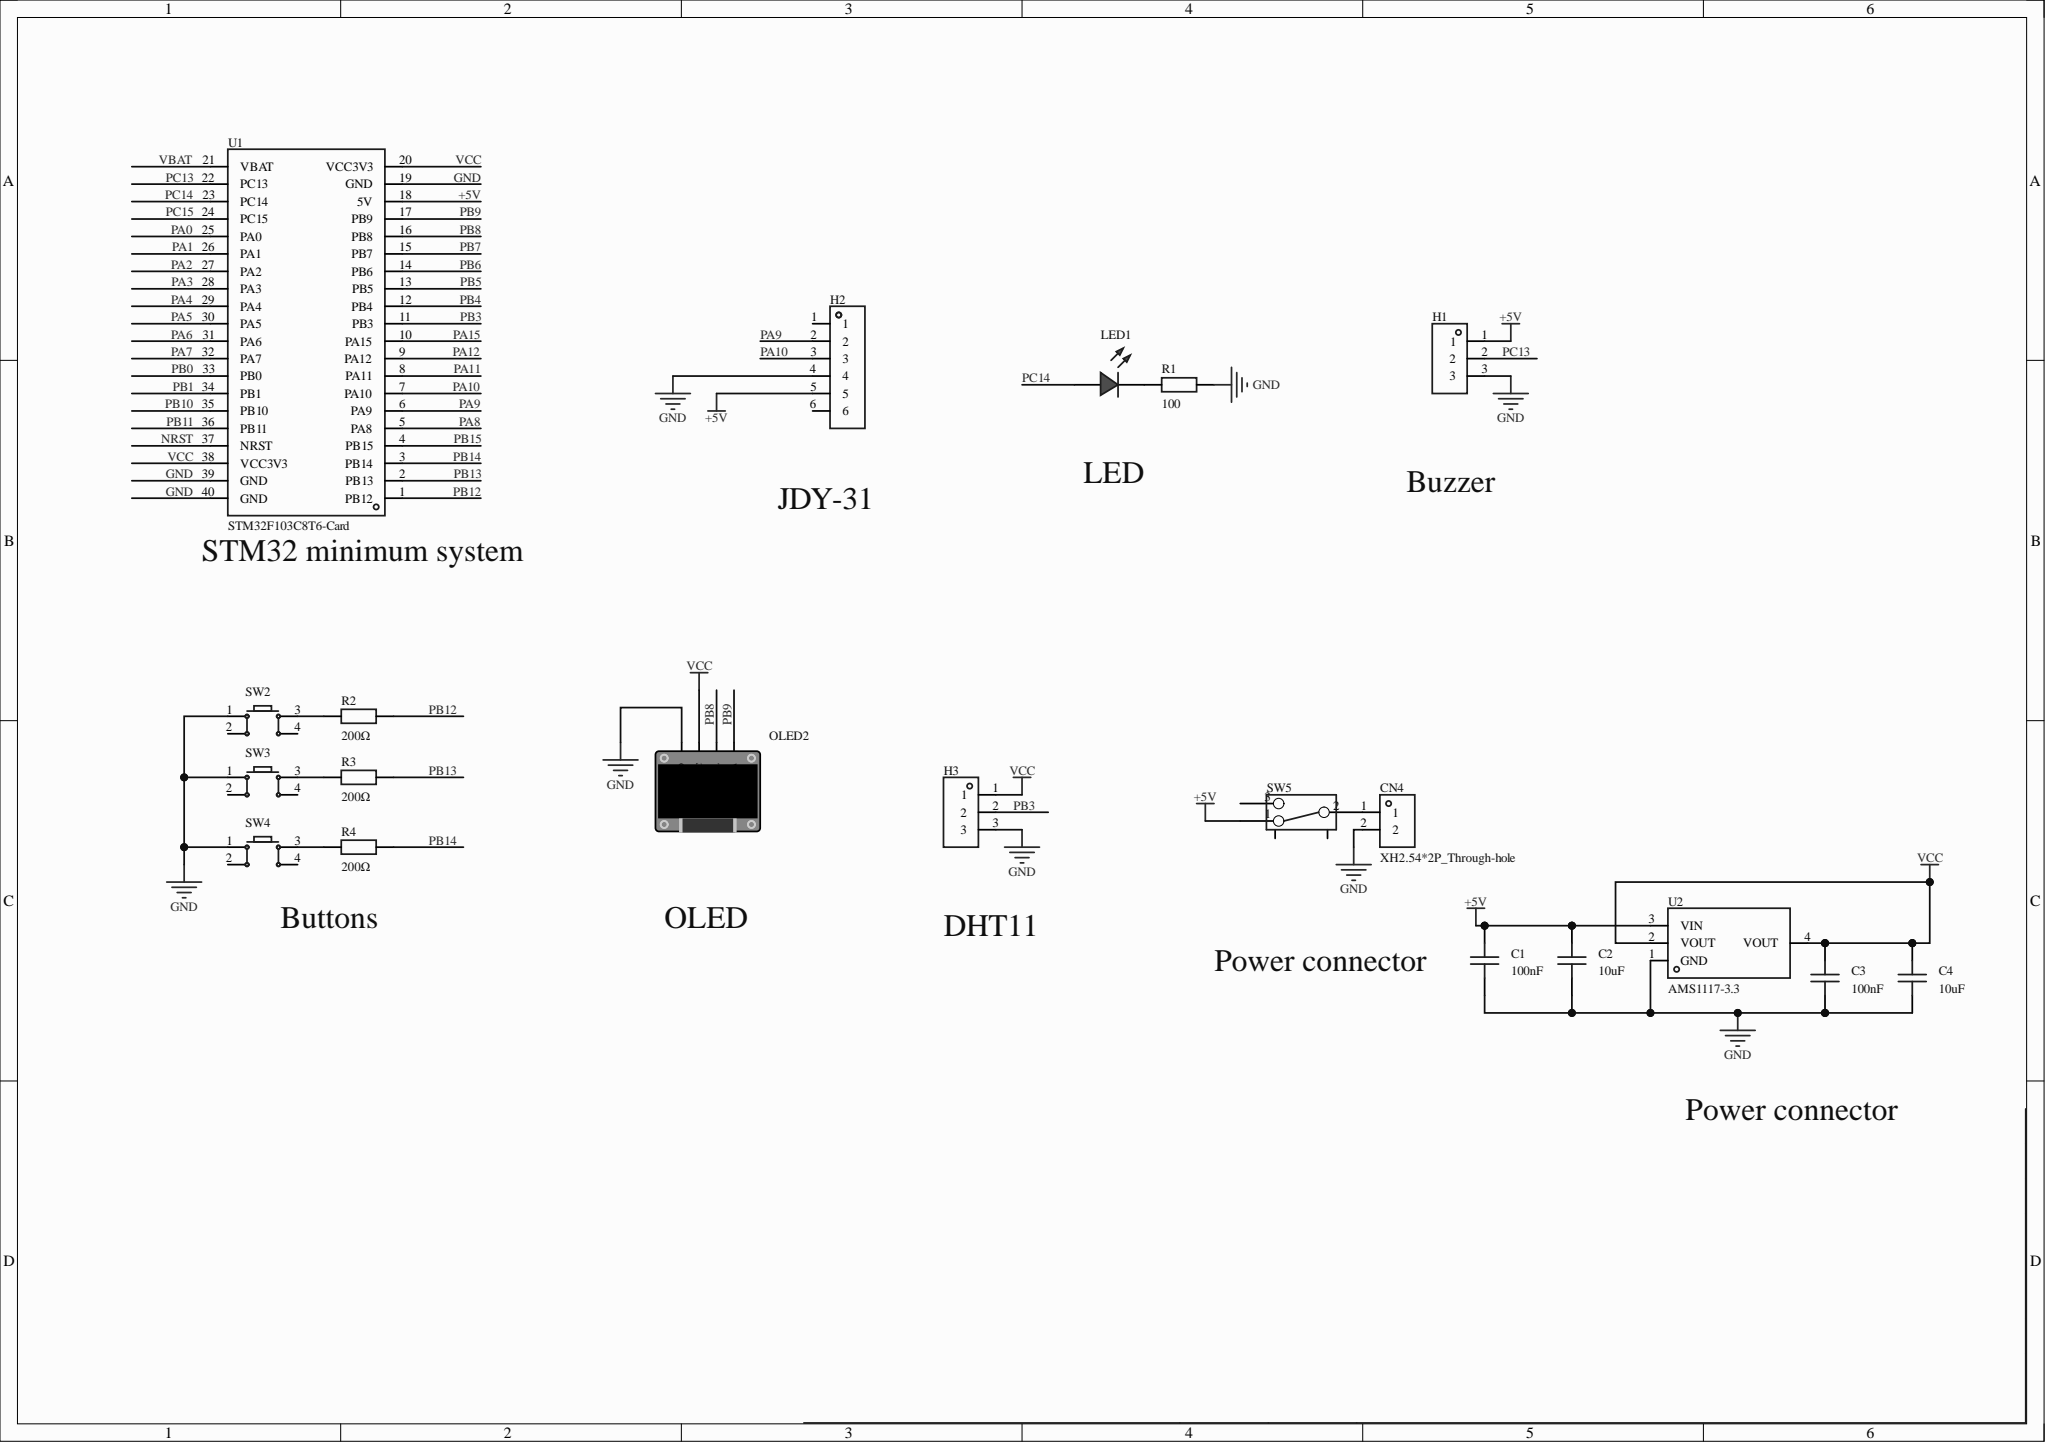Circuit board | Altium Designer | 20 parts | 18 nets
Bill of materials:
Comment,Description,Designator,Footprint,LibRef,Quantity
"100nF","","C1, C3","C0603","CAP_0603","2"
"10uF","","C2, C4","C0603","CAP_0603","2"
"XH2.54*2P_Through-hole","","CN4","CONN-TH_2P-P2.50-XH2.54-2P","XH2.54*2P_直插","1"
"","","H1, H3","HDR-TH_3P-P2.54-V-F","HDR-F_2.54_1x3P","2"
"","","H2","HDR-TH_6P-P2.54-V-F","HDR-F_2.54_1x6P","1"
"","","LED1","LED_TH-3mm","LED_TH-R_3mm","1"
"","","OLED2","0.96OLED_4P","0.96OLED模块_4P","1"
"100","","R1","Res_1/8W","Res_AXIAL-1/8W","1"
"200Ω","","R2, R3, R4","Res_1/8W","Res_AXIAL-1/8W","3"
"","","SW2, SW3, SW4","SW-TH_4P-L6.0-W6.0-P4.50-LS6.5","Key_TH_6x6x6","3"
"","","SW5","拨动开关","拨动开关_正","1"
"STM32F103C8T6-Card","","U1","CONN-TH_L53.3-W22.9_STM32F103C8T6-CARD","STM32F103C8T6-Card","1"
"AMS1117-3.3","Output type:Fixed;Operating voltage:-;Output voltage:3.3V;Output current:1A;Power supply ripple rejection ratio(PSRR):72dB@(120Hz);Output polarity:Positive;","U2","SOT-223-3_L6.5-W3.4-P2.30-LS7.0-BR","AMS1117-3.3_C6186","1"
Netlist (Protel format):
[
C1
C0603
100nF



]
[
C2
C0603
10uF



]
[
C3
C0603
100nF



]
[
C4
C0603
10uF



]
[
CN4
CONN-TH_2P-P2.50-XH2.54-2P
XH2.54*2P_Through-hole



]
[
H1
HDR-TH_3P-P2.54-V-F




]
[
H2
HDR-TH_6P-P2.54-V-F




]
[
H3
HDR-TH_3P-P2.54-V-F




]
[
LED1
LED_TH-3mm




]
[
OLED2
0.96OLED_4P




]
[
R1
Res_1/8W
100



]
[
R2
Res_1/8W
200Ω



]
[
R3
Res_1/8W
200Ω



]
[
R4
Res_1/8W
200Ω



]
[
SW2
SW-TH_4P-L6.0-W6.0-P4.50-LS6.5




]
[
SW3
SW-TH_4P-L6.0-W6.0-P4.50-LS6.5




]
[
SW4
SW-TH_4P-L6.0-W6.0-P4.50-LS6.5




]
[
SW5
拨动开关




]
[
U1
CONN-TH_L53.3-W22.9_STM32F103C8T6-CARD
STM32F103C8T6-Card



]
[
U2
SOT-223-3_L6.5-W3.4-P2.30-LS7.0-BR
AMS1117-3.3



]
(
VCC
C3-2
C4-2
H3-1
OLED2-2
U1-20
U1-38
U2-2
U2-4
)
(
PC14
LED1-1
U1-23
)
(
PC13
H1-2
U1-22
)
(
PB14
R4-2
U1-3
)
(
PB13
R3-2
U1-2
)
(
PB12
R2-2
U1-1
)
(
PB9
OLED2-4
U1-17
)
(
PB8
OLED2-3
U1-16
)
(
PB3
H3-2
U1-11
)
(
PA10
H2-3
U1-7
)
(
PA9
H2-2
U1-6
)
(
NetR4_1
R4-1
SW4-3
)
(
NetR3_1
R3-1
SW3-3
)
(
NetR2_1
R2-1
SW2-3
)
(
NetLED1_2
LED1-2
R1-1
)
(
NetCN4_1
CN4-1
SW5-2
)
(
GND
C1-1
C2-1
C3-1
C4-1
CN4-2
H1-3
H2-4
H3-3
OLED2-1
R1-2
SW2-1
SW3-1
SW4-1
U1-19
U1-39
U1-40
U2-1
)
(
+5V
C1-2
C2-2
H1-1
H2-5
SW5-1
U1-18
U2-3
)